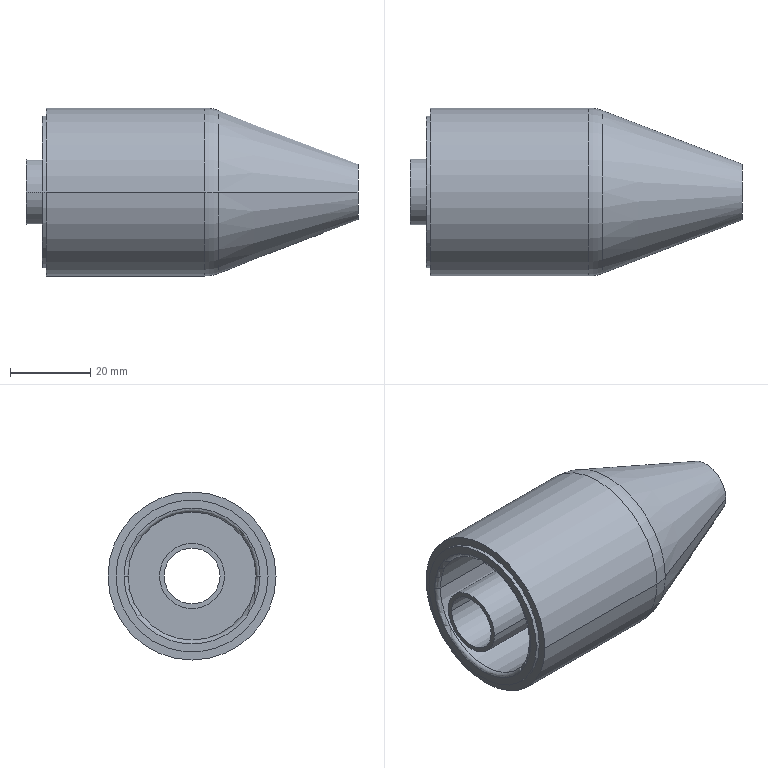Part | NX | features BREP 1 | 1 solid | 20 faces | box 83 x 42 x 42 mm | volume 45689 mm3 | cylinder 10 | torus 4 | plane 4 | cone 2 | commonest cylinder face diameters 14 x2 16.312 x2 32 x2 38 x2 42 x2
STEP:
#1=CARTESIAN_POINT('',(1.729,20.337,0.));
#2=VERTEX_POINT('',#1);
#3=CARTESIAN_POINT('',(-1.852,21.,0.));
#4=VERTEX_POINT('',#3);
#5=CARTESIAN_POINT('',(-1.852,11.,0.));
#6=DIRECTION('',(0.,0.,-1.));
#7=DIRECTION('',(0.,1.,0.));
#8=AXIS2_PLACEMENT_3D('',#5,#6,#7);
#9=CIRCLE('',#8,10.);
#10=EDGE_CURVE('',#2,#4,#9,.F.);
#11=ORIENTED_EDGE('',*,*,#10,.T.);
#12=CARTESIAN_POINT('',(-1.852,-21.,0.));
#13=VERTEX_POINT('',#12);
#14=CARTESIAN_POINT('',(-1.852,0.,0.));
#15=DIRECTION('',(1.,0.,0.));
#16=DIRECTION('',(0.,1.,0.));
#17=AXIS2_PLACEMENT_3D('',#14,#15,#16);
#18=CIRCLE('',#17,21.);
#19=EDGE_CURVE('',#4,#13,#18,.T.);
#20=ORIENTED_EDGE('',*,*,#19,.T.);
#21=CARTESIAN_POINT('',(1.729,-20.337,0.));
#22=VERTEX_POINT('',#21);
#23=CARTESIAN_POINT('',(-1.852,-11.,0.));
#24=DIRECTION('',(0.,0.,1.));
#25=DIRECTION('',(0.,-1.,0.));
#26=AXIS2_PLACEMENT_3D('',#23,#24,#25);
#27=CIRCLE('',#26,10.);
#28=EDGE_CURVE('',#22,#13,#27,.F.);
#29=ORIENTED_EDGE('',*,*,#28,.F.);
#30=CARTESIAN_POINT('',(1.729,0.,0.));
#31=DIRECTION('',(-1.,0.,0.));
#32=DIRECTION('',(0.,-1.,0.));
#33=AXIS2_PLACEMENT_3D('',#30,#31,#32);
#34=CIRCLE('',#33,20.337);
#35=EDGE_CURVE('',#22,#2,#34,.T.);
#36=ORIENTED_EDGE('',*,*,#35,.T.);
#37=EDGE_LOOP('',(#11,#20,#29,#36));
#38=FACE_BOUND('',#37,.T.);
#39=CARTESIAN_POINT('',(-1.852,0.,0.));
#40=DIRECTION('',(-1.,0.,0.));
#41=DIRECTION('',(0.,-1.,0.));
#42=AXIS2_PLACEMENT_3D('',#39,#40,#41);
#43=TOROIDAL_SURFACE('',#42,11.,10.);
#44=ADVANCED_FACE('',(#38),#43,.T.);
#45=CARTESIAN_POINT('',(36.5,7.,0.));
#46=VERTEX_POINT('',#45);
#47=CARTESIAN_POINT('',(1.729,20.337,0.));
#48=DIRECTION('',(0.9337,-0.3581,0.));
#49=VECTOR('',#48,1000.);
#50=LINE('',#47,#49);
#51=EDGE_CURVE('',#46,#2,#50,.F.);
#52=ORIENTED_EDGE('',*,*,#51,.T.);
#53=ORIENTED_EDGE('',*,*,#35,.F.);
#54=CARTESIAN_POINT('',(36.5,-7.,0.));
#55=VERTEX_POINT('',#54);
#56=CARTESIAN_POINT('',(1.729,-20.337,0.));
#57=DIRECTION('',(0.9337,0.3581,0.));
#58=VECTOR('',#57,1000.);
#59=LINE('',#56,#58);
#60=EDGE_CURVE('',#55,#22,#59,.F.);
#61=ORIENTED_EDGE('',*,*,#60,.F.);
#62=CARTESIAN_POINT('',(36.5,0.,0.));
#63=DIRECTION('',(-1.,0.,0.));
#64=DIRECTION('',(0.,-1.,0.));
#65=AXIS2_PLACEMENT_3D('',#62,#63,#64);
#66=CIRCLE('',#65,7.);
#67=EDGE_CURVE('',#55,#46,#66,.T.);
#68=ORIENTED_EDGE('',*,*,#67,.T.);
#69=EDGE_LOOP('',(#52,#53,#61,#68));
#70=FACE_BOUND('',#69,.T.);
#71=CARTESIAN_POINT('',(19.115,0.,0.));
#72=DIRECTION('',(-1.,0.,0.));
#73=DIRECTION('',(0.,-1.,0.));
#74=AXIS2_PLACEMENT_3D('',#71,#72,#73);
#75=CONICAL_SURFACE('',#74,13.668,0.3663);
#76=ADVANCED_FACE('',(#70),#75,.T.);
#77=CARTESIAN_POINT('',(-46.5,7.,0.));
#78=VERTEX_POINT('',#77);
#79=CARTESIAN_POINT('',(-46.5,-7.,0.));
#80=VERTEX_POINT('',#79);
#81=CARTESIAN_POINT('',(-46.5,0.,0.));
#82=DIRECTION('',(1.,0.,0.));
#83=DIRECTION('',(0.,1.,0.));
#84=AXIS2_PLACEMENT_3D('',#81,#82,#83);
#85=CIRCLE('',#84,7.);
#86=EDGE_CURVE('',#78,#80,#85,.T.);
#87=ORIENTED_EDGE('',*,*,#86,.F.);
#88=CARTESIAN_POINT('',(36.5,7.,0.));
#89=DIRECTION('',(-1.,0.,0.));
#90=VECTOR('',#89,1000.);
#91=LINE('',#88,#90);
#92=EDGE_CURVE('',#78,#46,#91,.F.);
#93=ORIENTED_EDGE('',*,*,#92,.T.);
#94=ORIENTED_EDGE('',*,*,#67,.F.);
#95=CARTESIAN_POINT('',(36.5,-7.,0.));
#96=DIRECTION('',(-1.,0.,0.));
#97=VECTOR('',#96,1000.);
#98=LINE('',#95,#97);
#99=EDGE_CURVE('',#80,#55,#98,.F.);
#100=ORIENTED_EDGE('',*,*,#99,.F.);
#101=EDGE_LOOP('',(#87,#93,#94,#100));
#102=FACE_BOUND('',#101,.T.);
#103=CARTESIAN_POINT('',(0.,0.,0.));
#104=DIRECTION('',(1.,0.,0.));
#105=DIRECTION('',(0.,1.,0.));
#106=AXIS2_PLACEMENT_3D('',#103,#104,#105);
#107=CYLINDRICAL_SURFACE('',#106,7.);
#108=ADVANCED_FACE('',(#102),#107,.F.);
#109=ORIENTED_EDGE('',*,*,#99,.T.);
#110=CARTESIAN_POINT('',(36.5,0.,0.));
#111=DIRECTION('',(-1.,0.,0.));
#112=DIRECTION('',(0.,1.,0.));
#113=AXIS2_PLACEMENT_3D('',#110,#111,#112);
#114=CIRCLE('',#113,7.);
#115=EDGE_CURVE('',#46,#55,#114,.T.);
#116=ORIENTED_EDGE('',*,*,#115,.F.);
#117=ORIENTED_EDGE('',*,*,#92,.F.);
#118=CARTESIAN_POINT('',(-46.5,0.,0.));
#119=DIRECTION('',(1.,0.,0.));
#120=DIRECTION('',(0.,-1.,0.));
#121=AXIS2_PLACEMENT_3D('',#118,#119,#120);
#122=CIRCLE('',#121,7.);
#123=EDGE_CURVE('',#80,#78,#122,.T.);
#124=ORIENTED_EDGE('',*,*,#123,.F.);
#125=EDGE_LOOP('',(#109,#116,#117,#124));
#126=FACE_BOUND('',#125,.T.);
#127=CARTESIAN_POINT('',(0.,0.,0.));
#128=DIRECTION('',(1.,0.,0.));
#129=DIRECTION('',(0.,1.,0.));
#130=AXIS2_PLACEMENT_3D('',#127,#128,#129);
#131=CYLINDRICAL_SURFACE('',#130,7.);
#132=ADVANCED_FACE('',(#126),#131,.F.);
#133=CARTESIAN_POINT('',(-46.5,8.156,0.));
#134=VERTEX_POINT('',#133);
#135=CARTESIAN_POINT('',(-46.5,-8.156,0.));
#136=VERTEX_POINT('',#135);
#137=CARTESIAN_POINT('',(-46.5,0.,0.));
#138=DIRECTION('',(-1.,0.,0.));
#139=DIRECTION('',(0.,1.,0.));
#140=AXIS2_PLACEMENT_3D('',#137,#138,#139);
#141=CIRCLE('',#140,8.156);
#142=EDGE_CURVE('',#134,#136,#141,.T.);
#143=ORIENTED_EDGE('',*,*,#142,.T.);
#144=CARTESIAN_POINT('',(-46.5,0.,0.));
#145=DIRECTION('',(-1.,0.,0.));
#146=DIRECTION('',(0.,-1.,0.));
#147=AXIS2_PLACEMENT_3D('',#144,#145,#146);
#148=CIRCLE('',#147,8.156);
#149=EDGE_CURVE('',#136,#134,#148,.T.);
#150=ORIENTED_EDGE('',*,*,#149,.T.);
#151=EDGE_LOOP('',(#143,#150));
#152=FACE_BOUND('',#151,.T.);
#153=ORIENTED_EDGE('',*,*,#123,.T.);
#154=ORIENTED_EDGE('',*,*,#86,.T.);
#155=EDGE_LOOP('',(#153,#154));
#156=FACE_BOUND('',#155,.T.);
#157=CARTESIAN_POINT('',(-46.5,8.156,0.));
#158=DIRECTION('',(-1.,0.,0.));
#159=DIRECTION('',(0.,0.,1.));
#160=AXIS2_PLACEMENT_3D('',#157,#158,#159);
#161=PLANE('',#160);
#162=ADVANCED_FACE('',(#152,#156),#161,.T.);
#163=CARTESIAN_POINT('',(0.,-8.156,0.));
#164=VERTEX_POINT('',#163);
#165=CARTESIAN_POINT('',(0.,-8.156,0.));
#166=DIRECTION('',(-1.,0.,0.));
#167=VECTOR('',#166,1000.);
#168=LINE('',#165,#167);
#169=EDGE_CURVE('',#164,#136,#168,.T.);
#170=ORIENTED_EDGE('',*,*,#169,.F.);
#171=CARTESIAN_POINT('',(0.,8.156,0.));
#172=VERTEX_POINT('',#171);
#173=CARTESIAN_POINT('',(0.,0.,0.));
#174=DIRECTION('',(1.,0.,0.));
#175=DIRECTION('',(0.,1.,0.));
#176=AXIS2_PLACEMENT_3D('',#173,#174,#175);
#177=CIRCLE('',#176,8.156);
#178=EDGE_CURVE('',#172,#164,#177,.T.);
#179=ORIENTED_EDGE('',*,*,#178,.F.);
#180=CARTESIAN_POINT('',(0.,8.156,0.));
#181=DIRECTION('',(-1.,0.,0.));
#182=VECTOR('',#181,1000.);
#183=LINE('',#180,#182);
#184=EDGE_CURVE('',#172,#134,#183,.T.);
#185=ORIENTED_EDGE('',*,*,#184,.T.);
#186=ORIENTED_EDGE('',*,*,#149,.F.);
#187=EDGE_LOOP('',(#170,#179,#185,#186));
#188=FACE_BOUND('',#187,.T.);
#189=CARTESIAN_POINT('',(0.,0.,0.));
#190=DIRECTION('',(1.,0.,0.));
#191=DIRECTION('',(0.,1.,0.));
#192=AXIS2_PLACEMENT_3D('',#189,#190,#191);
#193=CYLINDRICAL_SURFACE('',#192,8.156);
#194=ADVANCED_FACE('',(#188),#193,.T.);
#195=ORIENTED_EDGE('',*,*,#142,.F.);
#196=ORIENTED_EDGE('',*,*,#184,.F.);
#197=CARTESIAN_POINT('',(0.,0.,0.));
#198=DIRECTION('',(1.,0.,0.));
#199=DIRECTION('',(0.,-1.,0.));
#200=AXIS2_PLACEMENT_3D('',#197,#198,#199);
#201=CIRCLE('',#200,8.156);
#202=EDGE_CURVE('',#164,#172,#201,.T.);
#203=ORIENTED_EDGE('',*,*,#202,.F.);
#204=ORIENTED_EDGE('',*,*,#169,.T.);
#205=EDGE_LOOP('',(#195,#196,#203,#204));
#206=FACE_BOUND('',#205,.T.);
#207=CARTESIAN_POINT('',(0.,0.,0.));
#208=DIRECTION('',(1.,0.,0.));
#209=DIRECTION('',(0.,1.,0.));
#210=AXIS2_PLACEMENT_3D('',#207,#208,#209);
#211=CYLINDRICAL_SURFACE('',#210,8.156);
#212=ADVANCED_FACE('',(#206),#211,.T.);
#213=CARTESIAN_POINT('',(0.,16.,0.));
#214=VERTEX_POINT('',#213);
#215=CARTESIAN_POINT('',(0.,-16.,0.));
#216=VERTEX_POINT('',#215);
#217=CARTESIAN_POINT('',(0.,0.,0.));
#218=DIRECTION('',(-1.,0.,0.));
#219=DIRECTION('',(0.,1.,0.));
#220=AXIS2_PLACEMENT_3D('',#217,#218,#219);
#221=CIRCLE('',#220,16.);
#222=EDGE_CURVE('',#214,#216,#221,.T.);
#223=ORIENTED_EDGE('',*,*,#222,.T.);
#224=CARTESIAN_POINT('',(0.,0.,0.));
#225=DIRECTION('',(-1.,0.,0.));
#226=DIRECTION('',(0.,-1.,0.));
#227=AXIS2_PLACEMENT_3D('',#224,#225,#226);
#228=CIRCLE('',#227,16.);
#229=EDGE_CURVE('',#216,#214,#228,.T.);
#230=ORIENTED_EDGE('',*,*,#229,.T.);
#231=EDGE_LOOP('',(#223,#230));
#232=FACE_BOUND('',#231,.T.);
#233=ORIENTED_EDGE('',*,*,#202,.T.);
#234=ORIENTED_EDGE('',*,*,#178,.T.);
#235=EDGE_LOOP('',(#233,#234));
#236=FACE_BOUND('',#235,.T.);
#237=CARTESIAN_POINT('',(0.,8.156,0.));
#238=DIRECTION('',(-1.,0.,0.));
#239=DIRECTION('',(0.,0.,1.));
#240=AXIS2_PLACEMENT_3D('',#237,#238,#239);
#241=PLANE('',#240);
#242=ADVANCED_FACE('',(#232,#236),#241,.T.);
#243=CARTESIAN_POINT('',(-41.5,16.,0.));
#244=VERTEX_POINT('',#243);
#245=CARTESIAN_POINT('',(-41.5,-16.,0.));
#246=VERTEX_POINT('',#245);
#247=CARTESIAN_POINT('',(-41.5,0.,0.));
#248=DIRECTION('',(1.,0.,0.));
#249=DIRECTION('',(0.,1.,0.));
#250=AXIS2_PLACEMENT_3D('',#247,#248,#249);
#251=CIRCLE('',#250,16.);
#252=EDGE_CURVE('',#244,#246,#251,.T.);
#253=ORIENTED_EDGE('',*,*,#252,.F.);
#254=CARTESIAN_POINT('',(0.,16.,0.));
#255=DIRECTION('',(-1.,0.,0.));
#256=VECTOR('',#255,1000.);
#257=LINE('',#254,#256);
#258=EDGE_CURVE('',#244,#214,#257,.F.);
#259=ORIENTED_EDGE('',*,*,#258,.T.);
#260=ORIENTED_EDGE('',*,*,#229,.F.);
#261=CARTESIAN_POINT('',(0.,-16.,0.));
#262=DIRECTION('',(-1.,0.,0.));
#263=VECTOR('',#262,1000.);
#264=LINE('',#261,#263);
#265=EDGE_CURVE('',#246,#216,#264,.F.);
#266=ORIENTED_EDGE('',*,*,#265,.F.);
#267=EDGE_LOOP('',(#253,#259,#260,#266));
#268=FACE_BOUND('',#267,.T.);
#269=CARTESIAN_POINT('',(0.,0.,0.));
#270=DIRECTION('',(1.,0.,0.));
#271=DIRECTION('',(0.,1.,0.));
#272=AXIS2_PLACEMENT_3D('',#269,#270,#271);
#273=CYLINDRICAL_SURFACE('',#272,16.);
#274=ADVANCED_FACE('',(#268),#273,.F.);
#275=ORIENTED_EDGE('',*,*,#265,.T.);
#276=ORIENTED_EDGE('',*,*,#222,.F.);
#277=ORIENTED_EDGE('',*,*,#258,.F.);
#278=CARTESIAN_POINT('',(-41.5,0.,0.));
#279=DIRECTION('',(1.,0.,0.));
#280=DIRECTION('',(0.,-1.,0.));
#281=AXIS2_PLACEMENT_3D('',#278,#279,#280);
#282=CIRCLE('',#281,16.);
#283=EDGE_CURVE('',#246,#244,#282,.T.);
#284=ORIENTED_EDGE('',*,*,#283,.F.);
#285=EDGE_LOOP('',(#275,#276,#277,#284));
#286=FACE_BOUND('',#285,.T.);
#287=CARTESIAN_POINT('',(0.,0.,0.));
#288=DIRECTION('',(1.,0.,0.));
#289=DIRECTION('',(0.,1.,0.));
#290=AXIS2_PLACEMENT_3D('',#287,#288,#289);
#291=CYLINDRICAL_SURFACE('',#290,16.);
#292=ADVANCED_FACE('',(#286),#291,.F.);
#293=CARTESIAN_POINT('',(-42.5,-17.,0.));
#294=VERTEX_POINT('',#293);
#295=CARTESIAN_POINT('',(-42.5,17.,0.));
#296=VERTEX_POINT('',#295);
#297=CARTESIAN_POINT('',(-42.5,0.,0.));
#298=DIRECTION('',(1.,0.,0.));
#299=DIRECTION('',(0.,-1.,0.));
#300=AXIS2_PLACEMENT_3D('',#297,#298,#299);
#301=CIRCLE('',#300,17.);
#302=EDGE_CURVE('',#294,#296,#301,.T.);
#303=ORIENTED_EDGE('',*,*,#302,.F.);
#304=CARTESIAN_POINT('',(-41.5,-17.,0.));
#305=DIRECTION('',(0.,0.,1.));
#306=DIRECTION('',(0.,1.,0.));
#307=AXIS2_PLACEMENT_3D('',#304,#305,#306);
#308=CIRCLE('',#307,1.);
#309=EDGE_CURVE('',#246,#294,#308,.T.);
#310=ORIENTED_EDGE('',*,*,#309,.F.);
#311=ORIENTED_EDGE('',*,*,#283,.T.);
#312=CARTESIAN_POINT('',(-41.5,17.,0.));
#313=DIRECTION('',(0.,0.,-1.));
#314=DIRECTION('',(0.,-1.,0.));
#315=AXIS2_PLACEMENT_3D('',#312,#313,#314);
#316=CIRCLE('',#315,1.);
#317=EDGE_CURVE('',#244,#296,#316,.T.);
#318=ORIENTED_EDGE('',*,*,#317,.T.);
#319=EDGE_LOOP('',(#303,#310,#311,#318));
#320=FACE_BOUND('',#319,.T.);
#321=CARTESIAN_POINT('',(-41.5,0.,0.));
#322=DIRECTION('',(-1.,0.,0.));
#323=DIRECTION('',(0.,-1.,0.));
#324=AXIS2_PLACEMENT_3D('',#321,#322,#323);
#325=TOROIDAL_SURFACE('',#324,17.,1.);
#326=ADVANCED_FACE('',(#320),#325,.T.);
#327=ORIENTED_EDGE('',*,*,#317,.F.);
#328=ORIENTED_EDGE('',*,*,#252,.T.);
#329=ORIENTED_EDGE('',*,*,#309,.T.);
#330=CARTESIAN_POINT('',(-42.5,0.,0.));
#331=DIRECTION('',(1.,0.,0.));
#332=DIRECTION('',(0.,1.,0.));
#333=AXIS2_PLACEMENT_3D('',#330,#331,#332);
#334=CIRCLE('',#333,17.);
#335=EDGE_CURVE('',#296,#294,#334,.T.);
#336=ORIENTED_EDGE('',*,*,#335,.F.);
#337=EDGE_LOOP('',(#327,#328,#329,#336));
#338=FACE_BOUND('',#337,.T.);
#339=CARTESIAN_POINT('',(-41.5,0.,0.));
#340=DIRECTION('',(-1.,0.,0.));
#341=DIRECTION('',(0.,-1.,0.));
#342=AXIS2_PLACEMENT_3D('',#339,#340,#341);
#343=TOROIDAL_SURFACE('',#342,17.,1.);
#344=ADVANCED_FACE('',(#338),#343,.T.);
#345=CARTESIAN_POINT('',(-42.5,19.,0.));
#346=VERTEX_POINT('',#345);
#347=CARTESIAN_POINT('',(-42.5,-19.,0.));
#348=VERTEX_POINT('',#347);
#349=CARTESIAN_POINT('',(-42.5,0.,0.));
#350=DIRECTION('',(-1.,0.,0.));
#351=DIRECTION('',(0.,1.,0.));
#352=AXIS2_PLACEMENT_3D('',#349,#350,#351);
#353=CIRCLE('',#352,19.);
#354=EDGE_CURVE('',#346,#348,#353,.T.);
#355=ORIENTED_EDGE('',*,*,#354,.T.);
#356=CARTESIAN_POINT('',(-42.5,0.,0.));
#357=DIRECTION('',(-1.,0.,0.));
#358=DIRECTION('',(0.,-1.,0.));
#359=AXIS2_PLACEMENT_3D('',#356,#357,#358);
#360=CIRCLE('',#359,19.);
#361=EDGE_CURVE('',#348,#346,#360,.T.);
#362=ORIENTED_EDGE('',*,*,#361,.T.);
#363=EDGE_LOOP('',(#355,#362));
#364=FACE_BOUND('',#363,.T.);
#365=ORIENTED_EDGE('',*,*,#335,.T.);
#366=ORIENTED_EDGE('',*,*,#302,.T.);
#367=EDGE_LOOP('',(#365,#366));
#368=FACE_BOUND('',#367,.T.);
#369=CARTESIAN_POINT('',(-42.5,19.,0.));
#370=DIRECTION('',(-1.,0.,0.));
#371=DIRECTION('',(0.,0.,1.));
#372=AXIS2_PLACEMENT_3D('',#369,#370,#371);
#373=PLANE('',#372);
#374=ADVANCED_FACE('',(#364,#368),#373,.T.);
#375=CARTESIAN_POINT('',(-41.5,-19.,0.));
#376=VERTEX_POINT('',#375);
#377=CARTESIAN_POINT('',(-41.5,-19.,0.));
#378=DIRECTION('',(-1.,0.,0.));
#379=VECTOR('',#378,1000.);
#380=LINE('',#377,#379);
#381=EDGE_CURVE('',#376,#348,#380,.T.);
#382=ORIENTED_EDGE('',*,*,#381,.F.);
#383=CARTESIAN_POINT('',(-41.5,19.,0.));
#384=VERTEX_POINT('',#383);
#385=CARTESIAN_POINT('',(-41.5,0.,0.));
#386=DIRECTION('',(1.,0.,0.));
#387=DIRECTION('',(0.,1.,0.));
#388=AXIS2_PLACEMENT_3D('',#385,#386,#387);
#389=CIRCLE('',#388,19.);
#390=EDGE_CURVE('',#384,#376,#389,.T.);
#391=ORIENTED_EDGE('',*,*,#390,.F.);
#392=CARTESIAN_POINT('',(-41.5,19.,0.));
#393=DIRECTION('',(-1.,0.,0.));
#394=VECTOR('',#393,1000.);
#395=LINE('',#392,#394);
#396=EDGE_CURVE('',#384,#346,#395,.T.);
#397=ORIENTED_EDGE('',*,*,#396,.T.);
#398=ORIENTED_EDGE('',*,*,#361,.F.);
#399=EDGE_LOOP('',(#382,#391,#397,#398));
#400=FACE_BOUND('',#399,.T.);
#401=CARTESIAN_POINT('',(0.,0.,0.));
#402=DIRECTION('',(1.,0.,0.));
#403=DIRECTION('',(0.,1.,0.));
#404=AXIS2_PLACEMENT_3D('',#401,#402,#403);
#405=CYLINDRICAL_SURFACE('',#404,19.);
#406=ADVANCED_FACE('',(#400),#405,.T.);
#407=ORIENTED_EDGE('',*,*,#354,.F.);
#408=ORIENTED_EDGE('',*,*,#396,.F.);
#409=CARTESIAN_POINT('',(-41.5,0.,0.));
#410=DIRECTION('',(1.,0.,0.));
#411=DIRECTION('',(0.,-1.,0.));
#412=AXIS2_PLACEMENT_3D('',#409,#410,#411);
#413=CIRCLE('',#412,19.);
#414=EDGE_CURVE('',#376,#384,#413,.T.);
#415=ORIENTED_EDGE('',*,*,#414,.F.);
#416=ORIENTED_EDGE('',*,*,#381,.T.);
#417=EDGE_LOOP('',(#407,#408,#415,#416));
#418=FACE_BOUND('',#417,.T.);
#419=CARTESIAN_POINT('',(0.,0.,0.));
#420=DIRECTION('',(1.,0.,0.));
#421=DIRECTION('',(0.,1.,0.));
#422=AXIS2_PLACEMENT_3D('',#419,#420,#421);
#423=CYLINDRICAL_SURFACE('',#422,19.);
#424=ADVANCED_FACE('',(#418),#423,.T.);
#425=CARTESIAN_POINT('',(-41.5,21.,0.));
#426=VERTEX_POINT('',#425);
#427=CARTESIAN_POINT('',(-41.5,-21.,0.));
#428=VERTEX_POINT('',#427);
#429=CARTESIAN_POINT('',(-41.5,0.,0.));
#430=DIRECTION('',(-1.,0.,0.));
#431=DIRECTION('',(0.,1.,0.));
#432=AXIS2_PLACEMENT_3D('',#429,#430,#431);
#433=CIRCLE('',#432,21.);
#434=EDGE_CURVE('',#426,#428,#433,.T.);
#435=ORIENTED_EDGE('',*,*,#434,.T.);
#436=CARTESIAN_POINT('',(-41.5,0.,0.));
#437=DIRECTION('',(-1.,0.,0.));
#438=DIRECTION('',(0.,-1.,0.));
#439=AXIS2_PLACEMENT_3D('',#436,#437,#438);
#440=CIRCLE('',#439,21.);
#441=EDGE_CURVE('',#428,#426,#440,.T.);
#442=ORIENTED_EDGE('',*,*,#441,.T.);
#443=EDGE_LOOP('',(#435,#442));
#444=FACE_BOUND('',#443,.T.);
#445=ORIENTED_EDGE('',*,*,#414,.T.);
#446=ORIENTED_EDGE('',*,*,#390,.T.);
#447=EDGE_LOOP('',(#445,#446));
#448=FACE_BOUND('',#447,.T.);
#449=CARTESIAN_POINT('',(-41.5,19.,0.));
#450=DIRECTION('',(-1.,0.,0.));
#451=DIRECTION('',(0.,0.,1.));
#452=AXIS2_PLACEMENT_3D('',#449,#450,#451);
#453=PLANE('',#452);
#454=ADVANCED_FACE('',(#444,#448),#453,.T.);
#455=CARTESIAN_POINT('',(-1.852,-21.,0.));
#456=DIRECTION('',(-1.,0.,0.));
#457=VECTOR('',#456,1000.);
#458=LINE('',#455,#457);
#459=EDGE_CURVE('',#13,#428,#458,.T.);
#460=ORIENTED_EDGE('',*,*,#459,.F.);
#461=ORIENTED_EDGE('',*,*,#19,.F.);
#462=CARTESIAN_POINT('',(-1.852,21.,0.));
#463=DIRECTION('',(-1.,0.,0.));
#464=VECTOR('',#463,1000.);
#465=LINE('',#462,#464);
#466=EDGE_CURVE('',#4,#426,#465,.T.);
#467=ORIENTED_EDGE('',*,*,#466,.T.);
#468=ORIENTED_EDGE('',*,*,#441,.F.);
#469=EDGE_LOOP('',(#460,#461,#467,#468));
#470=FACE_BOUND('',#469,.T.);
#471=CARTESIAN_POINT('',(0.,0.,0.));
#472=DIRECTION('',(1.,0.,0.));
#473=DIRECTION('',(0.,1.,0.));
#474=AXIS2_PLACEMENT_3D('',#471,#472,#473);
#475=CYLINDRICAL_SURFACE('',#474,21.);
#476=ADVANCED_FACE('',(#470),#475,.T.);
#477=ORIENTED_EDGE('',*,*,#434,.F.);
#478=ORIENTED_EDGE('',*,*,#466,.F.);
#479=CARTESIAN_POINT('',(-1.852,0.,0.));
#480=DIRECTION('',(1.,0.,0.));
#481=DIRECTION('',(0.,-1.,0.));
#482=AXIS2_PLACEMENT_3D('',#479,#480,#481);
#483=CIRCLE('',#482,21.);
#484=EDGE_CURVE('',#13,#4,#483,.T.);
#485=ORIENTED_EDGE('',*,*,#484,.F.);
#486=ORIENTED_EDGE('',*,*,#459,.T.);
#487=EDGE_LOOP('',(#477,#478,#485,#486));
#488=FACE_BOUND('',#487,.T.);
#489=CARTESIAN_POINT('',(0.,0.,0.));
#490=DIRECTION('',(1.,0.,0.));
#491=DIRECTION('',(0.,1.,0.));
#492=AXIS2_PLACEMENT_3D('',#489,#490,#491);
#493=CYLINDRICAL_SURFACE('',#492,21.);
#494=ADVANCED_FACE('',(#488),#493,.T.);
#495=CARTESIAN_POINT('',(1.729,0.,0.));
#496=DIRECTION('',(-1.,0.,0.));
#497=DIRECTION('',(0.,1.,0.));
#498=AXIS2_PLACEMENT_3D('',#495,#496,#497);
#499=CIRCLE('',#498,20.337);
#500=EDGE_CURVE('',#2,#22,#499,.T.);
#501=ORIENTED_EDGE('',*,*,#500,.T.);
#502=ORIENTED_EDGE('',*,*,#28,.T.);
#503=ORIENTED_EDGE('',*,*,#484,.T.);
#504=ORIENTED_EDGE('',*,*,#10,.F.);
#505=EDGE_LOOP('',(#501,#502,#503,#504));
#506=FACE_BOUND('',#505,.T.);
#507=CARTESIAN_POINT('',(-1.852,0.,0.));
#508=DIRECTION('',(-1.,0.,0.));
#509=DIRECTION('',(0.,-1.,0.));
#510=AXIS2_PLACEMENT_3D('',#507,#508,#509);
#511=TOROIDAL_SURFACE('',#510,11.,10.);
#512=ADVANCED_FACE('',(#506),#511,.T.);
#513=ORIENTED_EDGE('',*,*,#115,.T.);
#514=ORIENTED_EDGE('',*,*,#60,.T.);
#515=ORIENTED_EDGE('',*,*,#500,.F.);
#516=ORIENTED_EDGE('',*,*,#51,.F.);
#517=EDGE_LOOP('',(#513,#514,#515,#516));
#518=FACE_BOUND('',#517,.T.);
#519=CARTESIAN_POINT('',(19.115,0.,0.));
#520=DIRECTION('',(-1.,0.,0.));
#521=DIRECTION('',(0.,-1.,0.));
#522=AXIS2_PLACEMENT_3D('',#519,#520,#521);
#523=CONICAL_SURFACE('',#522,13.668,0.3663);
#524=ADVANCED_FACE('',(#518),#523,.T.);
#525=CLOSED_SHELL('',(#44,#76,#108,#132,#162,#194,#212,#242,#274,#292,#326,#344,#374,#406,#424,#454,#476,#494,#512,#524));
#526=MANIFOLD_SOLID_BREP('',#525);
#527=(LENGTH_UNIT()NAMED_UNIT(*)SI_UNIT(.MILLI.,.METRE.));
#528=UNCERTAINTY_MEASURE_WITH_UNIT(LENGTH_MEASURE(0.00001),#527,'','');
#529=(NAMED_UNIT(*)PLANE_ANGLE_UNIT()SI_UNIT($,.RADIAN.));
#530=(NAMED_UNIT(*)SI_UNIT($,.STERADIAN.)SOLID_ANGLE_UNIT());
#531=(GEOMETRIC_REPRESENTATION_CONTEXT(3)GLOBAL_UNCERTAINTY_ASSIGNED_CONTEXT((#528))GLOBAL_UNIT_ASSIGNED_CONTEXT((#527,#529,#530))REPRESENTATION_CONTEXT('',''));
#532=ADVANCED_BREP_SHAPE_REPRESENTATION('',(#526),#531);